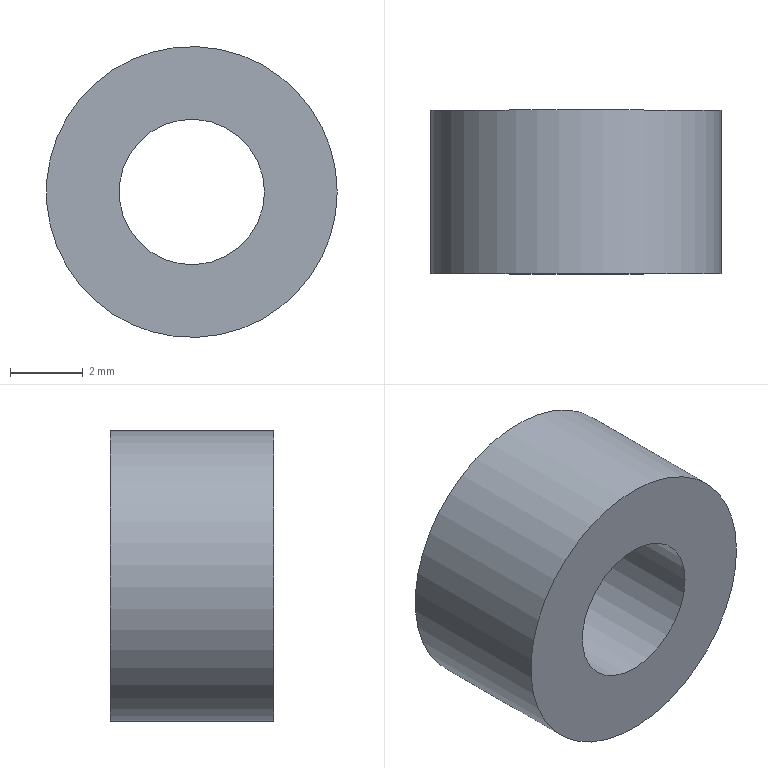Part | STEP file | 1-06.5 | 1 solid | 4 faces | box 8 x 4.5 x 8 mm | volume 169.646 mm3 | plane 2 | cylinder 2 | commonest cylinder face diameters 4 x1 8 x1
STEP:
#1=CARTESIAN_POINT('',(0.,0.,0.));
#2=DIRECTION('',(0.,0.,1.));
#3=DIRECTION('',(1.,0.,0.));
#4=AXIS2_PLACEMENT_3D('',#1,#2,#3);
#5=CARTESIAN_POINT('',(4.,0.,0.));
#6=VERTEX_POINT('',#5);
#7=CARTESIAN_POINT('',(0.,0.,0.));
#8=DIRECTION('',(0.,-1.,0.));
#9=DIRECTION('',(1.,0.,0.));
#10=AXIS2_PLACEMENT_3D('',#7,#8,#9);
#11=CIRCLE('',#10,4.);
#12=CARTESIAN_POINT('',(-1.072,0.,0.));
#13=DIRECTION('',(0.,-1.,0.));
#14=DIRECTION('',(1.,0.,0.));
#15=AXIS2_PLACEMENT_3D('',#12,#13,#14);
#16=PLANE('',#15);
#17=CARTESIAN_POINT('',(1.072,0.));
#18=DIRECTION('',(1.,0.));
#19=AXIS2_PLACEMENT_2D('',#17,#18);
#20=CIRCLE('',#19,4.);
#21=(GEOMETRIC_REPRESENTATION_CONTEXT(2)PARAMETRIC_REPRESENTATION_CONTEXT()REPRESENTATION_CONTEXT('',''));
#22=DEFINITIONAL_REPRESENTATION('',(#20),#21);
#23=PCURVE('',#16,#22);
#24=CARTESIAN_POINT('',(0.,0.,0.));
#25=DIRECTION('',(0.,1.,0.));
#26=DIRECTION('',(1.,0.,0.));
#27=AXIS2_PLACEMENT_3D('',#24,#25,#26);
#28=CYLINDRICAL_SURFACE('',#27,4.);
#29=CARTESIAN_POINT('',(6.283,0.));
#30=DIRECTION('',(-1.,0.));
#31=VECTOR('',#30,1.);
#32=LINE('',#29,#31);
#33=(GEOMETRIC_REPRESENTATION_CONTEXT(2)PARAMETRIC_REPRESENTATION_CONTEXT()REPRESENTATION_CONTEXT('',''));
#34=DEFINITIONAL_REPRESENTATION('',(#32),#33);
#35=PCURVE('',#28,#34);
#36=SURFACE_CURVE('',#11,(#23,#35),.PCURVE_S1.);
#37=EDGE_CURVE('',#6,#6,#36,.T.);
#38=ORIENTED_EDGE('',*,*,#37,.T.);
#39=EDGE_LOOP('',(#38));
#40=FACE_BOUND('',#39,.T.);
#41=CARTESIAN_POINT('',(2.,0.,0.));
#42=VERTEX_POINT('',#41);
#43=CARTESIAN_POINT('',(0.,0.,0.));
#44=DIRECTION('',(0.,1.,0.));
#45=DIRECTION('',(1.,0.,0.));
#46=AXIS2_PLACEMENT_3D('',#43,#44,#45);
#47=CIRCLE('',#46,2.);
#48=CARTESIAN_POINT('',(3.072,0.));
#49=CARTESIAN_POINT('',(3.072,-3.464));
#50=CARTESIAN_POINT('',(0.0718,-1.732));
#51=CARTESIAN_POINT('',(-2.928,0.));
#52=CARTESIAN_POINT('',(0.0718,1.732));
#53=CARTESIAN_POINT('',(3.072,3.464));
#54=CARTESIAN_POINT('',(3.072,0.));
#55=(BOUNDED_CURVE()B_SPLINE_CURVE(2,(#48,#49,#50,#51,#52,#53,#54),.UNSPECIFIED.,.T.,.F.)B_SPLINE_CURVE_WITH_KNOTS((1,2,2,2,2,1),(-2.094,0.,2.094,4.189,6.283,8.378),.UNSPECIFIED.)CURVE()GEOMETRIC_REPRESENTATION_ITEM()RATIONAL_B_SPLINE_CURVE((1.,0.5,1.,0.5,1.,0.5,1.))REPRESENTATION_ITEM(''));
#56=(GEOMETRIC_REPRESENTATION_CONTEXT(2)PARAMETRIC_REPRESENTATION_CONTEXT()REPRESENTATION_CONTEXT('',''));
#57=DEFINITIONAL_REPRESENTATION('',(#55),#56);
#58=PCURVE('',#16,#57);
#59=CARTESIAN_POINT('',(0.,0.,0.));
#60=DIRECTION('',(0.,1.,0.));
#61=DIRECTION('',(1.,0.,0.));
#62=AXIS2_PLACEMENT_3D('',#59,#60,#61);
#63=CYLINDRICAL_SURFACE('',#62,2.);
#64=CARTESIAN_POINT('',(0.,0.));
#65=DIRECTION('',(1.,0.));
#66=VECTOR('',#65,1.);
#67=LINE('',#64,#66);
#68=(GEOMETRIC_REPRESENTATION_CONTEXT(2)PARAMETRIC_REPRESENTATION_CONTEXT()REPRESENTATION_CONTEXT('',''));
#69=DEFINITIONAL_REPRESENTATION('',(#67),#68);
#70=PCURVE('',#63,#69);
#71=SURFACE_CURVE('',#47,(#58,#70),.PCURVE_S1.);
#72=EDGE_CURVE('',#42,#42,#71,.T.);
#73=ORIENTED_EDGE('',*,*,#72,.T.);
#74=EDGE_LOOP('',(#73));
#75=FACE_BOUND('',#74,.T.);
#76=ADVANCED_FACE('',(#40,#75),#16,.T.);
#77=CARTESIAN_POINT('',(4.,4.5,0.));
#78=VERTEX_POINT('',#77);
#79=CARTESIAN_POINT('',(0.,4.5,0.));
#80=DIRECTION('',(0.,-1.,0.));
#81=DIRECTION('',(1.,0.,0.));
#82=AXIS2_PLACEMENT_3D('',#79,#80,#81);
#83=CIRCLE('',#82,4.);
#84=CARTESIAN_POINT('',(-1.072,4.5,0.));
#85=DIRECTION('',(0.,-1.,0.));
#86=DIRECTION('',(1.,0.,0.));
#87=AXIS2_PLACEMENT_3D('',#84,#85,#86);
#88=PLANE('',#87);
#89=CARTESIAN_POINT('',(1.072,0.));
#90=DIRECTION('',(1.,0.));
#91=AXIS2_PLACEMENT_2D('',#89,#90);
#92=CIRCLE('',#91,4.);
#93=(GEOMETRIC_REPRESENTATION_CONTEXT(2)PARAMETRIC_REPRESENTATION_CONTEXT()REPRESENTATION_CONTEXT('',''));
#94=DEFINITIONAL_REPRESENTATION('',(#92),#93);
#95=PCURVE('',#88,#94);
#96=CARTESIAN_POINT('',(6.283,4.5));
#97=DIRECTION('',(-1.,0.));
#98=VECTOR('',#97,1.);
#99=LINE('',#96,#98);
#100=(GEOMETRIC_REPRESENTATION_CONTEXT(2)PARAMETRIC_REPRESENTATION_CONTEXT()REPRESENTATION_CONTEXT('',''));
#101=DEFINITIONAL_REPRESENTATION('',(#99),#100);
#102=PCURVE('',#28,#101);
#103=SURFACE_CURVE('',#83,(#95,#102),.PCURVE_S1.);
#104=EDGE_CURVE('',#78,#78,#103,.T.);
#105=ORIENTED_EDGE('',*,*,#104,.T.);
#106=EDGE_LOOP('',(#105));
#107=FACE_BOUND('',#106,.F.);
#108=CARTESIAN_POINT('',(2.,4.5,0.));
#109=VERTEX_POINT('',#108);
#110=CARTESIAN_POINT('',(0.,4.5,0.));
#111=DIRECTION('',(0.,1.,0.));
#112=DIRECTION('',(1.,0.,0.));
#113=AXIS2_PLACEMENT_3D('',#110,#111,#112);
#114=CIRCLE('',#113,2.);
#115=CARTESIAN_POINT('',(3.072,0.));
#116=CARTESIAN_POINT('',(3.072,-3.464));
#117=CARTESIAN_POINT('',(0.0718,-1.732));
#118=CARTESIAN_POINT('',(-2.928,0.));
#119=CARTESIAN_POINT('',(0.0718,1.732));
#120=CARTESIAN_POINT('',(3.072,3.464));
#121=CARTESIAN_POINT('',(3.072,0.));
#122=(BOUNDED_CURVE()B_SPLINE_CURVE(2,(#115,#116,#117,#118,#119,#120,#121),.UNSPECIFIED.,.T.,.F.)B_SPLINE_CURVE_WITH_KNOTS((1,2,2,2,2,1),(-2.094,0.,2.094,4.189,6.283,8.378),.UNSPECIFIED.)CURVE()GEOMETRIC_REPRESENTATION_ITEM()RATIONAL_B_SPLINE_CURVE((1.,0.5,1.,0.5,1.,0.5,1.))REPRESENTATION_ITEM(''));
#123=(GEOMETRIC_REPRESENTATION_CONTEXT(2)PARAMETRIC_REPRESENTATION_CONTEXT()REPRESENTATION_CONTEXT('',''));
#124=DEFINITIONAL_REPRESENTATION('',(#122),#123);
#125=PCURVE('',#88,#124);
#126=CARTESIAN_POINT('',(0.,4.5));
#127=DIRECTION('',(1.,0.));
#128=VECTOR('',#127,1.);
#129=LINE('',#126,#128);
#130=(GEOMETRIC_REPRESENTATION_CONTEXT(2)PARAMETRIC_REPRESENTATION_CONTEXT()REPRESENTATION_CONTEXT('',''));
#131=DEFINITIONAL_REPRESENTATION('',(#129),#130);
#132=PCURVE('',#63,#131);
#133=SURFACE_CURVE('',#114,(#125,#132),.PCURVE_S1.);
#134=EDGE_CURVE('',#109,#109,#133,.T.);
#135=ORIENTED_EDGE('',*,*,#134,.T.);
#136=EDGE_LOOP('',(#135));
#137=FACE_BOUND('',#136,.F.);
#138=ADVANCED_FACE('',(#107,#137),#88,.F.);
#139=CARTESIAN_POINT('',(4.,0.,0.));
#140=DIRECTION('',(0.,1.,0.));
#141=VECTOR('',#140,1.);
#142=LINE('',#139,#141);
#143=CARTESIAN_POINT('',(6.283,0.));
#144=DIRECTION('',(0.,1.));
#145=VECTOR('',#144,1.);
#146=LINE('',#143,#145);
#147=(GEOMETRIC_REPRESENTATION_CONTEXT(2)PARAMETRIC_REPRESENTATION_CONTEXT()REPRESENTATION_CONTEXT('',''));
#148=DEFINITIONAL_REPRESENTATION('',(#146),#147);
#149=PCURVE('',#28,#148);
#150=CARTESIAN_POINT('',(0.,0.));
#151=DIRECTION('',(0.,1.));
#152=VECTOR('',#151,1.);
#153=LINE('',#150,#152);
#154=(GEOMETRIC_REPRESENTATION_CONTEXT(2)PARAMETRIC_REPRESENTATION_CONTEXT()REPRESENTATION_CONTEXT('',''));
#155=DEFINITIONAL_REPRESENTATION('',(#153),#154);
#156=PCURVE('',#28,#155);
#157=SEAM_CURVE('',#142,(#149,#156),.PCURVE_S1.);
#158=EDGE_CURVE('',#6,#78,#157,.T.);
#159=ORIENTED_EDGE('',*,*,#158,.T.);
#160=ORIENTED_EDGE('',*,*,#104,.T.);
#161=ORIENTED_EDGE('',*,*,#158,.F.);
#162=ORIENTED_EDGE('',*,*,#37,.F.);
#163=EDGE_LOOP('',(#159,#160,#161,#162));
#164=FACE_BOUND('',#163,.T.);
#165=ADVANCED_FACE('',(#164),#28,.T.);
#166=ORIENTED_EDGE('',*,*,#72,.T.);
#167=CARTESIAN_POINT('',(2.,0.,0.));
#168=DIRECTION('',(0.,1.,0.));
#169=VECTOR('',#168,1.);
#170=LINE('',#167,#169);
#171=CARTESIAN_POINT('',(6.283,0.));
#172=DIRECTION('',(0.,1.));
#173=VECTOR('',#172,1.);
#174=LINE('',#171,#173);
#175=(GEOMETRIC_REPRESENTATION_CONTEXT(2)PARAMETRIC_REPRESENTATION_CONTEXT()REPRESENTATION_CONTEXT('',''));
#176=DEFINITIONAL_REPRESENTATION('',(#174),#175);
#177=PCURVE('',#63,#176);
#178=CARTESIAN_POINT('',(0.,0.));
#179=DIRECTION('',(0.,1.));
#180=VECTOR('',#179,1.);
#181=LINE('',#178,#180);
#182=(GEOMETRIC_REPRESENTATION_CONTEXT(2)PARAMETRIC_REPRESENTATION_CONTEXT()REPRESENTATION_CONTEXT('',''));
#183=DEFINITIONAL_REPRESENTATION('',(#181),#182);
#184=PCURVE('',#63,#183);
#185=SEAM_CURVE('',#170,(#177,#184),.PCURVE_S1.);
#186=EDGE_CURVE('',#42,#109,#185,.T.);
#187=ORIENTED_EDGE('',*,*,#186,.T.);
#188=ORIENTED_EDGE('',*,*,#134,.F.);
#189=ORIENTED_EDGE('',*,*,#186,.F.);
#190=EDGE_LOOP('',(#166,#187,#188,#189));
#191=FACE_BOUND('',#190,.F.);
#192=ADVANCED_FACE('',(#191),#63,.F.);
#193=CLOSED_SHELL('',(#76,#138,#165,#192));
#194=MANIFOLD_SOLID_BREP('',#193);
#195=(LENGTH_UNIT()NAMED_UNIT(*)SI_UNIT(.MILLI.,.METRE.));
#196=UNCERTAINTY_MEASURE_WITH_UNIT(LENGTH_MEASURE(0.0000001),#195,'','');
#197=(NAMED_UNIT(*)PLANE_ANGLE_UNIT()SI_UNIT($,.RADIAN.));
#198=(NAMED_UNIT(*)SI_UNIT($,.STERADIAN.)SOLID_ANGLE_UNIT());
#199=(GEOMETRIC_REPRESENTATION_CONTEXT(3)GLOBAL_UNCERTAINTY_ASSIGNED_CONTEXT((#196))GLOBAL_UNIT_ASSIGNED_CONTEXT((#195,#197,#198))REPRESENTATION_CONTEXT('',''));
#200=ADVANCED_BREP_SHAPE_REPRESENTATION('',(#4,#194),#199);